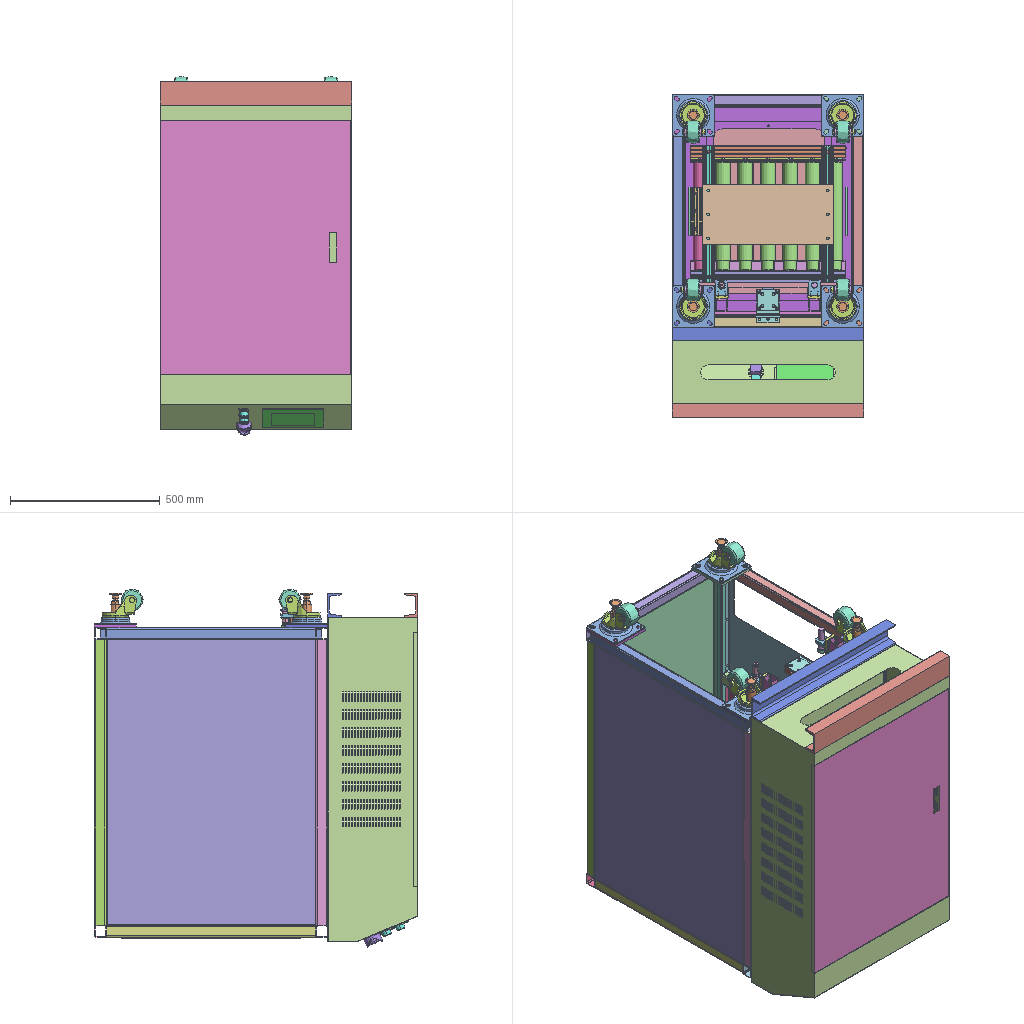Assembly | STEP file | 52 different items | 143 placed | box 640 x 1080 x 1198 mm
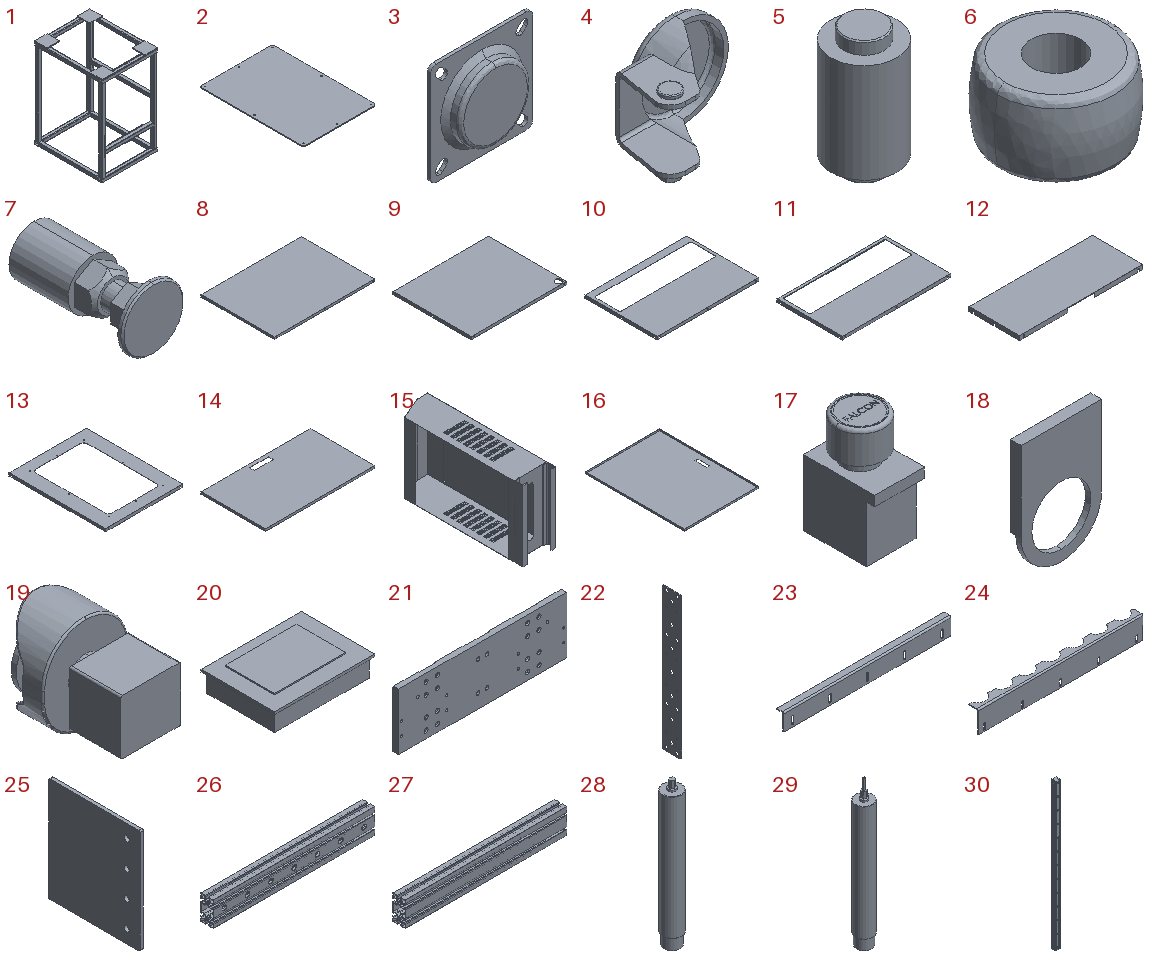Parts list (item | name | quantity | parent item | size | volume):
1 | PN_0029 | x1 | in PN_0031 | 640 x 780 x 1045 mm | 4745237 mm3
2 | PN_0012 | x1 | in PN_0031 | 420 x 600 x 5 mm | 1258440 mm3
3 | CDAN75-Ms | x4 | in CDAN75-M | 140 x 23.5 x 140 mm | 226200 mm3
4 | CDAN75-Mb | x4 | in CDAN75-M | 116 x 74 x 90 mm | 70869 mm3
5 | CDAN75-Mbe | x4 | in CDAN75-M | 30 x 30 x 56 mm | 34751 mm3
6 | CDAN75-Mw | x4 | in CDAN75-M | 75 x 74.925 x 45 mm | 156321 mm3
7 | CDAN75-Ma | x4 | in CDAN75-M | 40 x 77 x 40 mm | 48272 mm3
8 | PN_0009 | x1 | in PN_0031 | 955 x 698 x 20 mm | 728257 mm3
9 | PN_0008 | x1 | in PN_0031 | 683 x 558 x 20 mm | 425535 mm3
10 | PN_0006 | x1 | in PN_0031 | 698 x 493 x 20 mm | 273161 mm3
11 | PN_0003 | x1 | in PN_0031 | 698 x 418 x 20 mm | 217961 mm3
12 | PN_0020 | x1 | in PN_0031 | 558 x 228 x 20 mm | 153874 mm3
13 | PN_0017 | x1 | in PN_0031 | 558 x 698 x 20 mm | 233111 mm3
14 | PN_0019 | x1 | in PN_0031 | 953 x 560 x 20 mm | 584212 mm3
15 | PN_0027 | x1 | in PN_0031 | 300 x 1165 x 640 mm | 4220898 mm3
16 | PN_0010 | x1 | in PN_0031 | 636 x 850 x 15 mm | 579652 mm3
17 | Start unit | x2 | in PN_0031 | 30 x 43 x 65 mm | 60814 mm3
18 | Panel | x2 | in PN_0031 | 30 x 4 x 45 mm | 2788 mm3
19 | Component | x1 | in PN_0031 | 50 x 68 x 56 mm | 64949 mm3
20 | 7 inch screen | x1 | in PN_0031 | 204 x 150 x 45 mm | 1182850 mm3
21 | PN_0002 | x1 | in PN_0030 | 520 x 16 x 175 mm | 1376606 mm3
22 | PN_0021 | x2 | in PN_0030 | 3 x 70 x 520 mm | 101913 mm3
23 | PN_0016 | x1 | in PN_0030 | 470 x 20 x 48 mm | 59388 mm3
24 | PN_0022 | x1 | in PN_0030 | 520 x 30 x 70 mm | 90245 mm3
25 | PN_0023 | x2 | in PN_0030 | 5 x 140 x 160 mm | 110710 mm3
26 | PN_0025 | x1 | in PN_0030 | 520 x 40 x 80 mm | 382140 mm3
27 | PN_0024 | x1 | in PN_0030 | 520 x 40 x 80 mm | 378549 mm3
28 | Unpowered | x6 | in PN_0030 | 50.6 x 50.6 x 396 mm | 712589 mm3
29 | Electric roller | x1 | in PN_0030 | 50.6 x 50.6 x 426 mm | 713178 mm3
30 | HGH25 slide rail | x2 | in HGH25CA2R740Z0 | 23 x 22 x 740 mm | 310065 mm3
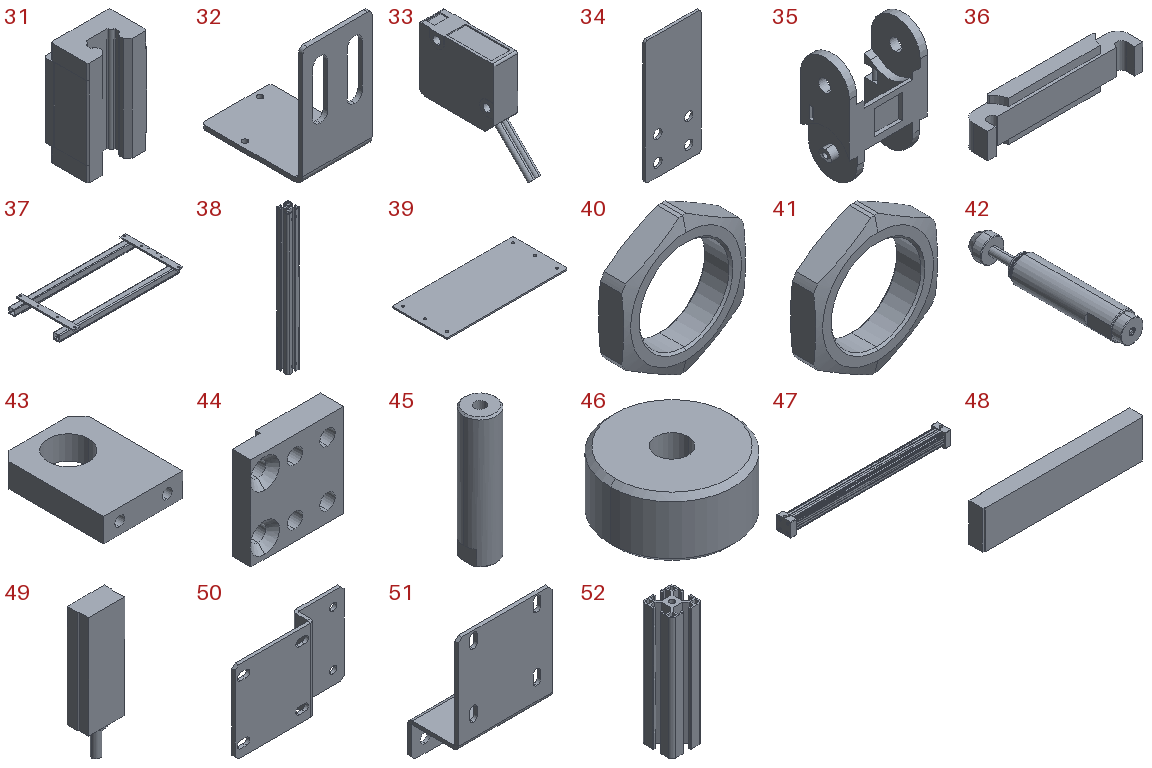31 | HGH25 slider | x4 | in HGH25CA2R740Z0 | 48 x 34.5 x 82 mm | 100220 mm3
32 | PN_0001 | x1 | in PN_0030 | 32 x 47 x 55 mm | 5577 mm3
33 | Connector switch | x1 | in PN_0030 | 10.4 x 45.161 x 39.591 mm | 8353 mm3
34 | PN_0013 | x1 | in PN_0030 | 45 x 2 x 100 mm | 8685 mm3
35 | MHPU203_30c | x25 | in MHPU203_30_MHPU203-30 | 32 x 20 x 45 mm | 6087 mm3
36 | MHPU203_30f | x25 | in MHPU203_30_MHPU203-30 | 27.6 x 4.5 x 7.143 mm | 492.21 mm3
37 | PN_0028 | x1 | in PN_0030 | 840 x 400 x 53 mm | 1080937 mm3
38 | PN_0004 | x2 | in PN_0030 | 40 x 40 x 458 mm | 262404 mm3
39 | PN_0011 | x1 | in PN_0030 | 440 x 200 x 5 mm | 437984 mm3
40 | ACA-2020-1 | x2 | in ACA-2020 | 26 x 6 x 29.132 mm | 1676 mm3
41 | ACA-2020-2 | x2 | in ACA-2020 | 26 x 6 x 29.132 mm | 1676 mm3
42 | ACA-2020-3 | x2 | in ACA-2020 | 20 x 118 x 20 mm | 28972 mm3
43 | PN_0014 | x5 | in PN_0030 | 40 x 53 x 12 mm | 20571 mm3
44 | PN_0026 | x5 | in PN_0030 | 40 x 10 x 40 mm | 12395 mm3
45 | PN_0032 | x2 | in PN_0030 | 20 x 20 x 80 mm | 24015 mm3
46 | PN_0007 | x2 | in PN_0030 | 25 x 25 x 12 mm | 5014 mm3
47 | HI_PRU40500b | x1 | in PRF40x500-S2_0_ | 800 x 69 x 69 mm | 2639652 mm3
48 | HI_PRF40500s | x1 | in PRF40x500-S2_0_ | 152 x 14 x 36 mm | 74599 mm3
49 | HI_S-CS-95 | x2 | in PRF40x500-S2_0_ | 10.9 x 7 x 39 mm | 1983 mm3
50 | PN_0005 | x1 | in PN_0030 | 115 x 18 x 75 mm | 27777 mm3
51 | PN_0015 | x1 | in PN_0030 | 80 x 43 x 110 mm | 34046 mm3
52 | PN_0018 | x1 | in PN_0030 | 40 x 40 x 160 mm | 89766 mm3
Placements (level | parent | child | x y z in mm | rotation matrix by rows):
1 | subassembly 2 | PN_0031 | -187.288 6.937 -27.35 | 1 0 0 0 1 0 0 0 1
2 | PN_0031 | PN_0029 | 410.985 15.607 562.0 | 1 0 0 0 1 0 0 0 1
2 | PN_0031 | PN_0012 | 203.735 -283.393 -459.0 | 1 0 0 0 1 0 0 0 1
2 | PN_0031 | CDAN75-M | 660.985 335.607 615.5 | 0 0 -1 1 0 0 0 -1 0
3 | CDAN75-M | CDAN75-Ms | -0.0 -0.0 -0.0 | 1 0 0 0 1 0 0 0 1
3 | CDAN75-M | CDAN75-Mb | -0.0 -0.0 -0.0 | 1 0 0 0 1 0 0 0 1
3 | CDAN75-M | CDAN75-Mbe | -0.0 -0.0 -0.0 | 1 0 0 0 1 0 0 0 1
3 | CDAN75-M | CDAN75-Mw | -0.0 -0.0 -0.0 | 1 0 0 0 1 0 0 0 1
3 | CDAN75-M | CDAN75-Ma | -0.0 -0.0 -0.0 | 1 0 0 0 1 0 0 0 1
2 | PN_0031 | CDAN75-M | 160.985 335.607 615.5 | 0 0 -1 1 0 0 0 -1 0
3 | CDAN75-M | CDAN75-Ms | -0.0 -0.0 -0.0 | 1 0 0 0 1 0 0 0 1
3 | CDAN75-M | CDAN75-Mb | -0.0 -0.0 -0.0 | 1 0 0 0 1 0 0 0 1
3 | CDAN75-M | CDAN75-Mbe | -0.0 -0.0 -0.0 | 1 0 0 0 1 0 0 0 1
3 | CDAN75-M | CDAN75-Mw | -0.0 -0.0 -0.0 | 1 0 0 0 1 0 0 0 1
3 | CDAN75-M | CDAN75-Ma | -0.0 -0.0 -0.0 | 1 0 0 0 1 0 0 0 1
2 | PN_0031 | CDAN75-M | 160.985 -304.393 615.5 | 0 0 1 -1 0 0 0 -1 0
3 | CDAN75-M | CDAN75-Ms | -0.0 -0.0 -0.0 | 1 0 0 0 1 0 0 0 1
3 | CDAN75-M | CDAN75-Mb | -0.0 -0.0 -0.0 | 1 0 0 0 1 0 0 0 1
3 | CDAN75-M | CDAN75-Mbe | -0.0 -0.0 -0.0 | 1 0 0 0 1 0 0 0 1
3 | CDAN75-M | CDAN75-Mw | -0.0 -0.0 -0.0 | 1 0 0 0 1 0 0 0 1
3 | CDAN75-M | CDAN75-Ma | -0.0 -0.0 -0.0 | 1 0 0 0 1 0 0 0 1
2 | PN_0031 | CDAN75-M | 660.985 -304.393 615.5 | 0 0 1 -1 0 0 0 -1 0
3 | CDAN75-M | CDAN75-Ms | -0.0 -0.0 -0.0 | 1 0 0 0 1 0 0 0 1
3 | CDAN75-M | CDAN75-Mb | -0.0 -0.0 -0.0 | 1 0 0 0 1 0 0 0 1
3 | CDAN75-M | CDAN75-Mbe | -0.0 -0.0 -0.0 | 1 0 0 0 1 0 0 0 1
3 | CDAN75-M | CDAN75-Mw | -0.0 -0.0 -0.0 | 1 0 0 0 1 0 0 0 1
3 | CDAN75-M | CDAN75-Ma | -0.0 -0.0 -0.0 | 1 0 0 0 1 0 0 0 1
2 | PN_0031 | PN_0009 | 110.985 -334.393 -413.0 | 0 0 -1 0 1 0 1 0 -0
2 | PN_0031 | PN_0008 | 690.985 -354.393 -141.0 | 0 -1 0 0 0 -1 1 0 -0
2 | PN_0031 | PN_0006 | 710.985 -332.393 -411.0 | 0 0 1 1 0 0 0 1 0
2 | PN_0031 | PN_0003 | 710.985 -332.393 124.0 | 0 0 1 1 0 0 0 1 -0
2 | PN_0031 | PN_0020 | 690.985 -354.393 -183.0 | -1 0 0 0 0 -1 0 -1 0
2 | PN_0031 | PN_0017 | 132.985 365.607 -434.0 | 1 0 0 0 -1 0 0 0 -1
2 | PN_0031 | PN_0019 | 690.985 385.607 542.0 | 0 -1 0 0 0 1 -1 0 0
2 | PN_0031 | PN_0027 | 730.985 -374.393 617.0 | 0 0 -1 1 0 0 0 -1 0
2 | PN_0031 | PN_0010 | 409.985 -674.393 141.0 | 1 0 0 0 0 1 0 -1 -0
2 | PN_0031 | Start unit | 370.985 -594.45 -366.994 | -0.999 0.04367 0 0.04019 0.9195 -0.3911 -0.01708 -0.3908 -0.9203
2 | PN_0031 | Start unit | 370.985 -548.433 -386.551 | -0.999 0.04367 0 0.04019 0.9195 -0.3911 -0.01708 -0.3908 -0.9203
2 | PN_0031 | Panel | 370.414 -619.325 -406.404 | -0.9971 0 -0.07621 0.07014 -0.3911 -0.9177 -0.02981 -0.9203 0.39
2 | PN_0031 | Panel | 370.414 -573.308 -425.961 | -0.9971 0 -0.07621 0.07014 -0.3911 -0.9177 -0.02981 -0.9203 0.39
2 | PN_0031 | Component | 370.755 -523.162 -447.273 | -0.997 0 -0.07687 0.07074 -0.3911 -0.9176 -0.03007 -0.9203 0.39
2 | PN_0031 | 7 inch screen | 534.985 -559.725 -390.988 | -1 0 0 0 0.9203 -0.3911 0 -0.3911 -0.9203
1 | subassembly 2 | PN_0030 | 303.86 -365.411 1.245 | 0 0 1 -1 0 0 0 -1 -0
2 | PN_0030 | PN_0002 | -147.955 36.01 -80.412 | 0 1 0 0 0 -1 -1 0 0
2 | PN_0030 | PN_0021 | -187.955 71.51 -340.412 | -1 0 0 0 1 0 0 0 -1
2 | PN_0030 | PN_0021 | -558.455 71.51 -340.412 | -1 0 0 0 1 0 0 0 -1
2 | PN_0030 | PN_0016 | -598.455 98.51 129.588 | 0 0 1 0 1 0 -1 0 -0
2 | PN_0030 | PN_0022 | -154.455 100.51 179.588 | 0 0 -1 0 -1 0 -1 0 0
2 | PN_0030 | PN_0023 | -307.455 -21.339 179.588 | 0 0 -1 0 1 0 1 0 0
2 | PN_0030 | PN_0025 | -585.955 78.51 -340.412 | 0 1 0 0 0 1 1 0 0
2 | PN_0030 | PN_0024 | -167.955 38.51 -340.412 | 0 -1 0 0 0 -1 1 0 -0
2 | PN_0030 | Unpowered | -222.455 58.76 -230.412 | 0 0 -1 0.3439 -0.939 0 -0.939 -0.3439 0
2 | PN_0030 | Unpowered | -222.455 58.76 144.588 | 0 0 -1 0.3439 -0.939 0 -0.939 -0.3439 0
2 | PN_0030 | Unpowered | -222.455 58.76 69.588 | 0 0 -1 0.3439 -0.939 0 -0.939 -0.3439 0
2 | PN_0030 | Unpowered | -222.455 58.76 -5.412 | 0 0 -1 0.3439 -0.939 0 -0.939 -0.3439 0
2 | PN_0030 | Unpowered | -222.455 58.76 -80.412 | 0 0 -1 0.3439 -0.939 0 -0.939 -0.3439 0
2 | PN_0030 | Unpowered | -222.455 58.76 -155.412 | 0 0 -1 0.3439 -0.939 0 -0.939 -0.3439 0
2 | PN_0030 | Electric roller | -222.455 58.361 -305.412 | 0 0 -1 0 1 0 1 0 0
2 | PN_0030 | HGH25CA2R740Z0 | -108.387 -214.405 -232.617 | 0 -1 0 0 0 1 -1 0 -0
3 | HGH25CA2R740Z0 | HGH25 slide rail | 4.046 -14.432 -225.0 | 1 0 0 0 1 0 0 0 1
3 | HGH25CA2R740Z0 | HGH25 slider | 4.046 -14.432 297.916 | 1 0 0 0 1 0 0 0 1
3 | HGH25CA2R740Z0 | HGH25 slider | 4.046 -14.432 202.916 | 1 0 0 0 1 0 0 0 1
2 | PN_0030 | HGH25CA2R740Z0 | -108.387 -214.405 80.383 | 0 -1 0 0 0 1 -1 0 -0
3 | HGH25CA2R740Z0 | HGH25 slide rail | 4.046 -14.432 -225.0 | 1 0 0 0 1 0 0 0 1
3 | HGH25CA2R740Z0 | HGH25 slider | 4.046 -14.432 297.916 | 1 0 0 0 1 0 0 0 1
3 | HGH25CA2R740Z0 | HGH25 slider | 4.046 -14.432 202.916 | 1 0 0 0 1 0 0 0 1
2 | PN_0030 | PN_0001 | -605.955 115.71 169.588 | 0 1 0 0 0 -1 -1 0 -0
2 | PN_0030 | Connector switch | -563.955 108.51 145.388 | 0 0 1 -1 0 0 0 -1 0
2 | PN_0030 | PN_0013 | -47.955 -410.405 53.338 | 0 -1 0 1 0 0 0 0 1
2 | PN_0030 | MHPU203_30_MHPU203-30 | -119.955 58.095 139.338 | 0 1 0 -1 0 0 0 0 1
3 | MHPU203_30_MHPU203-30 | MHPU203_30c | 32.5 -0.0 -0.0 | 0 0 1 0 1 0 -1 0 0
3 | MHPU203_30_MHPU203-30 | MHPU203_30f | 10.0 -0.0 -0.0 | 0 0 1 0 1 0 -1 0 0
3 | MHPU203_30_MHPU203-30 | MHPU203_30c | 7.067 -2.909 -0.0 | 0 0.2909 0.9567 0 0.9567 -0.2909 -1 0 -0
3 | MHPU203_30_MHPU203-30 | MHPU203_30f | -14.459 3.637 -0.0 | 0 0.2909 0.9567 0 0.9567 -0.2909 -1 0 -0
3 | MHPU203_30_MHPU203-30 | MHPU203_30c | -22.252 -1.817 -0.0 | 0 0.9091 0.4167 0 0.4167 -0.9091 -1 0 0
3 | MHPU203_30_MHPU203-30 | MHPU203_30f | -31.627 18.637 -0.0 | 0 0.9091 0.4167 0 0.4167 -0.9091 -1 0 0
3 | MHPU203_30_MHPU203-30 | MHPU203_30c | -41.002 20.909 -0.0 | 0 0.9091 -0.4167 0 -0.4167 -0.9091 -1 0 0
3 | MHPU203_30_MHPU203-30 | MHPU203_30f | -31.627 41.363 -0.0 | 0 0.9091 -0.4167 0 -0.4167 -0.9091 -1 0 0
3 | MHPU203_30_MHPU203-30 | MHPU203_30c | -35.986 49.817 -0.0 | 0 0.2909 -0.9567 0 -0.9567 -0.2909 -1 0 0
3 | MHPU203_30_MHPU203-30 | MHPU203_30f | -14.459 56.363 -0.0 | 0 0.2909 -0.9567 0 -0.9567 -0.2909 -1 0 0
3 | MHPU203_30_MHPU203-30 | MHPU203_30c | -12.5 60.0 -0.0 | 0 0 -1 0 -1 0 -1 0 0
3 | MHPU203_30_MHPU203-30 | MHPU203_30f | 10 60.0 -0.0 | 0 0 -1 0 -1 0 -1 0 0
3 | MHPU203_30_MHPU203-30 | MHPU203_30c | 12.5 60.0 -0.0 | 0 0 -1 0 -1 0 -1 0 0
3 | MHPU203_30_MHPU203-30 | MHPU203_30f | 35 60.0 -0.0 | 0 0 -1 0 -1 0 -1 0 0
3 | MHPU203_30_MHPU203-30 | MHPU203_30c | 37.5 60.0 -0.0 | 0 0 -1 0 -1 0 -1 0 0
3 | MHPU203_30_MHPU203-30 | MHPU203_30f | 60 60.0 -0.0 | 0 0 -1 0 -1 0 -1 0 0
3 | MHPU203_30_MHPU203-30 | MHPU203_30c | 62.5 60.0 -0.0 | 0 0 -1 0 -1 0 -1 0 0
3 | MHPU203_30_MHPU203-30 | MHPU203_30f | 85 60.0 -0.0 | 0 0 -1 0 -1 0 -1 0 0
3 | MHPU203_30_MHPU203-30 | MHPU203_30c | 87.5 60.0 -0.0 | 0 0 -1 0 -1 0 -1 0 0
3 | MHPU203_30_MHPU203-30 | MHPU203_30f | 110 60.0 -0.0 | 0 0 -1 0 -1 0 -1 0 0
3 | MHPU203_30_MHPU203-30 | MHPU203_30f | 135 60.0 -0.0 | 0 0 -1 0 -1 0 -1 0 0
3 | MHPU203_30_MHPU203-30 | MHPU203_30f | 160 60.0 -0.0 | 0 0 -1 0 -1 0 -1 0 0
3 | MHPU203_30_MHPU203-30 | MHPU203_30f | 185 60.0 -0.0 | 0 0 -1 0 -1 0 -1 0 0
3 | MHPU203_30_MHPU203-30 | MHPU203_30f | 210 60.0 -0.0 | 0 0 -1 0 -1 0 -1 0 0
3 | MHPU203_30_MHPU203-30 | MHPU203_30f | 235 60.0 -0.0 | 0 0 -1 0 -1 0 -1 0 0
3 | MHPU203_30_MHPU203-30 | MHPU203_30f | 260 60.0 -0.0 | 0 0 -1 0 -1 0 -1 0 0
3 | MHPU203_30_MHPU203-30 | MHPU203_30f | 285 60.0 -0.0 | 0 0 -1 0 -1 0 -1 0 0
3 | MHPU203_30_MHPU203-30 | MHPU203_30f | 310 60.0 -0.0 | 0 0 -1 0 -1 0 -1 0 0
3 | MHPU203_30_MHPU203-30 | MHPU203_30f | 335 60.0 -0.0 | 0 0 -1 0 -1 0 -1 0 0
3 | MHPU203_30_MHPU203-30 | MHPU203_30c | 112.5 60.0 -0.0 | 0 0 -1 0 -1 0 -1 0 0
3 | MHPU203_30_MHPU203-30 | MHPU203_30c | 137.5 60.0 -0.0 | 0 0 -1 0 -1 0 -1 0 0
3 | MHPU203_30_MHPU203-30 | MHPU203_30c | 162.5 60.0 -0.0 | 0 0 -1 0 -1 0 -1 0 0
3 | MHPU203_30_MHPU203-30 | MHPU203_30c | 187.5 60.0 -0.0 | 0 0 -1 0 -1 0 -1 0 0
3 | MHPU203_30_MHPU203-30 | MHPU203_30c | 212.5 60.0 -0.0 | 0 0 -1 0 -1 0 -1 0 0
3 | MHPU203_30_MHPU203-30 | MHPU203_30c | 237.5 60.0 -0.0 | 0 0 -1 0 -1 0 -1 0 0
3 | MHPU203_30_MHPU203-30 | MHPU203_30c | 262.5 60.0 -0.0 | 0 0 -1 0 -1 0 -1 0 0
3 | MHPU203_30_MHPU203-30 | MHPU203_30c | 287.5 60.0 -0.0 | 0 0 -1 0 -1 0 -1 0 0
3 | MHPU203_30_MHPU203-30 | MHPU203_30c | 312.5 60.0 -0.0 | 0 0 -1 0 -1 0 -1 0 0
3 | MHPU203_30_MHPU203-30 | MHPU203_30c | 57.5 -0.0 -0.0 | 0 0 1 0 1 0 -1 0 0
3 | MHPU203_30_MHPU203-30 | MHPU203_30f | 35.0 -0.0 -0.0 | 0 0 1 0 1 0 -1 0 0
3 | MHPU203_30_MHPU203-30 | MHPU203_30c | 337.5 60.0 -0.0 | 0 0 -1 0 -1 0 -1 0 0
3 | MHPU203_30_MHPU203-30 | MHPU203_30c | 362.5 60.0 -0.0 | 0 0 -1 0 -1 0 -1 0 0
3 | MHPU203_30_MHPU203-30 | MHPU203_30c | 387.5 60.0 -0.0 | 0 0 -1 0 -1 0 -1 0 0
3 | MHPU203_30_MHPU203-30 | MHPU203_30c | 412.5 60.0 -0.0 | 0 0 -1 0 -1 0 -1 0 0
3 | MHPU203_30_MHPU203-30 | MHPU203_30c | 437.5 60.0 -0.0 | 0 0 -1 0 -1 0 -1 0 0
3 | MHPU203_30_MHPU203-30 | MHPU203_30f | 360 60.0 -0.0 | 0 0 -1 0 -1 0 -1 0 0
3 | MHPU203_30_MHPU203-30 | MHPU203_30f | 385 60.0 -0.0 | 0 0 -1 0 -1 0 -1 0 0
3 | MHPU203_30_MHPU203-30 | MHPU203_30f | 410 60.0 -0.0 | 0 0 -1 0 -1 0 -1 0 0
3 | MHPU203_30_MHPU203-30 | MHPU203_30f | 435 60.0 -0.0 | 0 0 -1 0 -1 0 -1 0 0
3 | MHPU203_30_MHPU203-30 | MHPU203_30f | 460 60.0 -0.0 | 0 0 -1 0 -1 0 -1 0 0
2 | PN_0030 | PN_0028 | -70.955 -628.405 -235.162 | 0 0 1 1 0 0 0 1 -0
2 | PN_0030 | PN_0004 | -147.955 -1.49 -280.412 | 0 0 1 0 1 0 -1 0 -0
2 | PN_0030 | PN_0004 | -147.955 -1.49 119.588 | 0 0 1 0 1 0 -1 0 -0
2 | PN_0030 | PN_0011 | -476.955 -26.49 -300.412 | 0 1 0 0 0 1 1 0 -0
2 | PN_0030 | ACA-2020 | -139.955 -653.405 -235.162 | -0.9745 0 0.2243 0 1 0 -0.2243 0 -0.9745
3 | ACA-2020 | ACA-2020-1 | -0.0 -22.0 -0.0 | 0.9939 0 -0.11 0 1 0 0.11 0 0.9939
3 | ACA-2020 | ACA-2020-2 | 0.0 -2.0 -0.0 | 0.9756 0 0.2198 0 1 0 -0.2198 0 0.9756
3 | ACA-2020 | ACA-2020-3 | -0.0 -0.0 -0.0 | 1 0 0 0 1 0 0 0 1
2 | PN_0030 | PN_0014 | -101.955 -588.405 -255.162 | 0 -1 0 0 0 -1 1 0 -0
2 | PN_0030 | PN_0026 | -93.955 -588.405 -215.162 | 0 -1 0 -1 0 0 0 0 -1
2 | PN_0030 | PN_0026 | -93.955 171.595 -255.162 | 0 -1 0 1 0 0 0 0 1
2 | PN_0030 | PN_0014 | -101.955 183.595 -255.162 | 0 -1 0 0 0 -1 1 0 -0
2 | PN_0030 | ACA-2020 | -139.955 228.595 -235.162 | 0.9385 0 0.3453 0 -1 0 0.3453 0 -0.9385
3 | ACA-2020 | ACA-2020-1 | -0.0 -22.0 -0.0 | 0.9939 0 -0.11 0 1 0 0.11 0 0.9939
3 | ACA-2020 | ACA-2020-2 | 0.0 -2.0 -0.0 | 0.9756 0 0.2198 0 1 0 -0.2198 0 0.9756
3 | ACA-2020 | ACA-2020-3 | -0.0 -0.0 -0.0 | 1 0 0 0 1 0 0 0 1
2 | PN_0030 | PN_0026 | -93.955 171.595 54.838 | 0 -1 0 1 0 0 0 0 1
2 | PN_0030 | PN_0014 | -101.955 183.595 54.838 | 0 -1 0 0 0 -1 1 0 -0
2 | PN_0030 | PN_0032 | -139.955 234.595 74.838 | 1 0 0 0 0 -1 0 1 -0
2 | PN_0030 | PN_0032 | -139.955 -641.405 74.838 | 0.8372 0.5469 0 0 0 1 0.5469 -0.8372 -0
2 | PN_0030 | PN_0007 | -139.955 142.595 74.838 | 0.9237 0.383 0 0 0 1 0.383 -0.9237 0
2 | PN_0030 | PN_0007 | -139.955 -549.405 74.838 | 1 0 0 0 0 -1 0 1 0
2 | PN_0030 | PN_0014 | -101.955 -588.405 54.838 | 0 -1 0 0 0 -1 1 0 -0
2 | PN_0030 | PN_0026 | -93.955 -588.405 94.838 | 0 -1 0 -1 0 0 0 0 -1
2 | PN_0030 | PN_0026 | -93.955 171.595 54.838 | 0 -1 0 1 0 0 0 0 1
2 | PN_0030 | PN_0014 | -101.955 183.595 54.838 | 0 -1 0 0 0 -1 1 0 -0
2 | PN_0030 | PRF40x500-S2_0_ | -61.701 185.013 -59.225 | 0 -1 0 0 0 1 -1 0 0
3 | PRF40x500-S2_0_ | HI_PRU40500b | 20.938 -6.247 21.581 | 0 0 1 0 1 0 -1 0 0
3 | PRF40x500-S2_0_ | HI_PRF40500s | 20.938 58.253 -149.003 | 0 0 -1 0 1 0 1 0 -0
3 | PRF40x500-S2_0_ | HI_S-CS-95 | 28.1 35.4 -2.5 | 0 1 0 -1 0 0 0 0 1
3 | PRF40x500-S2_0_ | HI_S-CS-95 | 28.1 35.4 -741.5 | 0 1 0 1 0 0 0 0 -1
2 | PN_0030 | PN_0005 | -124.455 209.595 -117.662 | 1 0 0 0 1 0 0 0 1
2 | PN_0030 | PN_0015 | -124.455 -593.405 -120.162 | 0 0 -1 0 1 0 1 0 0
2 | PN_0030 | PN_0023 | -467.455 -21.339 -340.412 | 0 0 1 0 1 0 -1 0 -0
2 | PN_0030 | PN_0018 | -307.455 -1.49 -320.412 | 0 0 1 1 0 0 0 1 -0